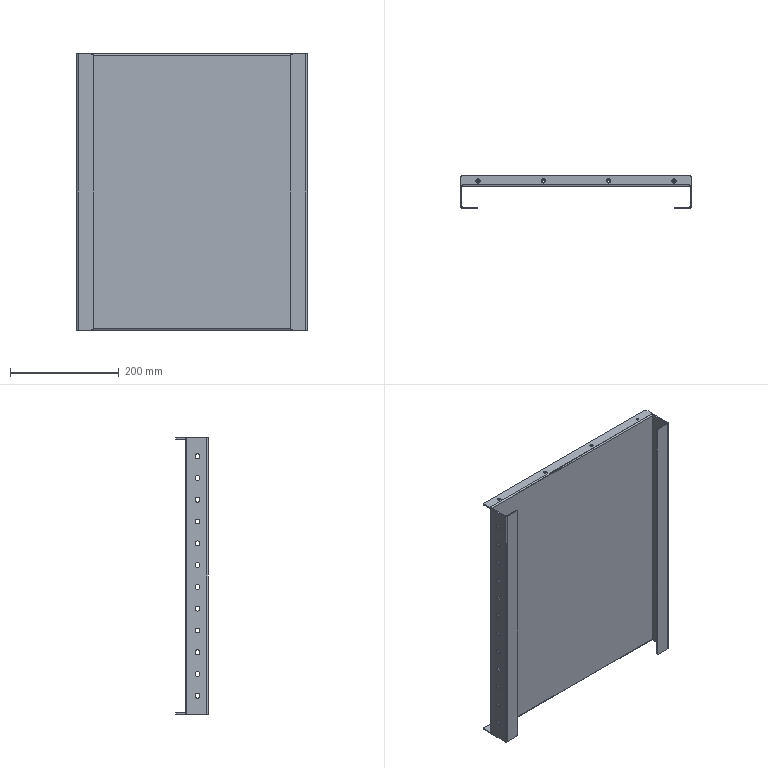Part | SolidWorks | features BreakCorner 3, ICE 2, SMBaseFlange 2, Chamfer 1, EdgeFlange 1, FlatPattern 1, LPattern 1, MirrorPattern 1, SheetMetal 1 | 1 solid | 152 faces | box 423 x 60 x 507 mm | volume 590095 mm3 | cylinder 84 | plane 52 | cone 16 | commonest cylinder face diameters 8.8 x48 5 x22 6 x8 1 x6